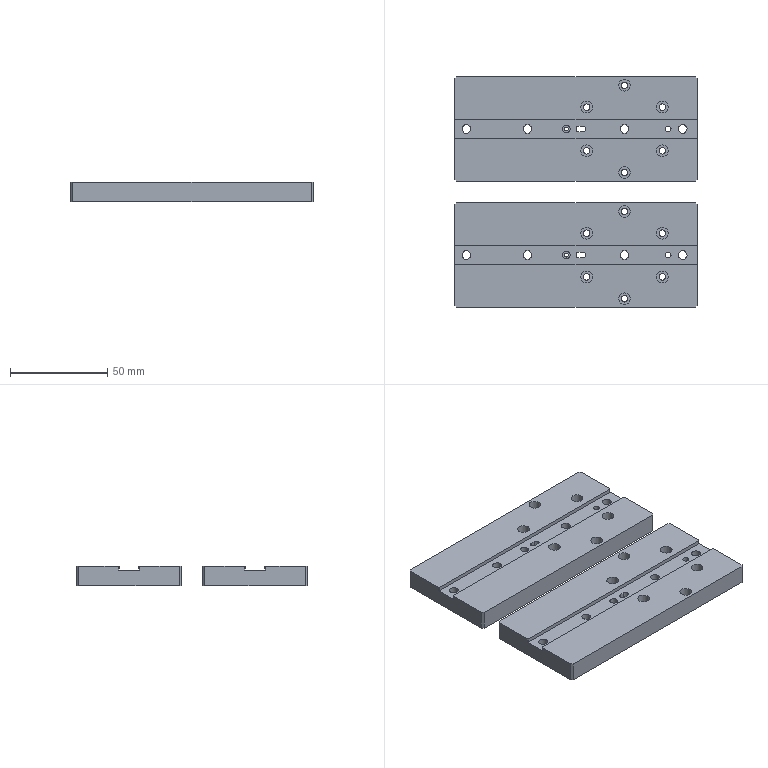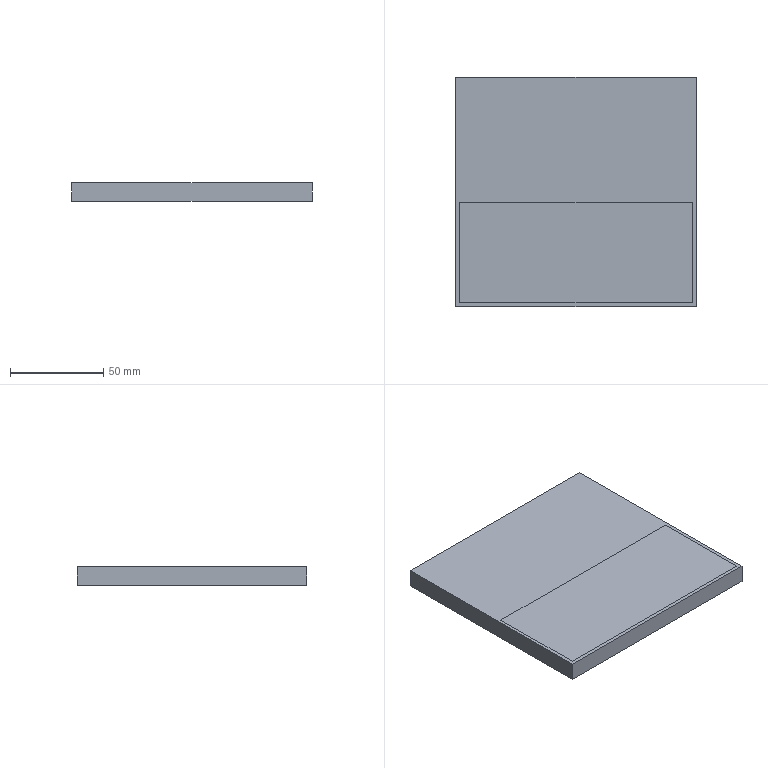CAM job | NX | 3-axis milling, drilling | part box 125 x 119 x 10 mm | stock box 129 x 123 x 10 mm
Tools:
number,name,description,diameter,corner_radius,flute_length,length,flutes
22,D6A45,Milling Tool-5 Parameters,6.0,0.0,3.0,3.0,2
20,D10,Milling Tool-5 Parameters,10.0,0.0,50.0,75.0,2
15,D4,Milling Tool-5 Parameters,4.0,0.0,50.0,75.0,2
13,D3,Milling Tool-5 Parameters,3.0,0.0,50.0,75.0,2
11,D10JING,Milling Tool-5 Parameters,10.0,0.0,50.0,75.0,2
19,4.5ZT,Drilling Tool,4.5,0.0,35.0,50.0,2
21,3.4ZT,Drilling Tool,3.4,0.0,35.0,50.0,2
24,2.0ZT,Drilling Tool,2.0,0.0,35.0,50.0,2
17,D6,Milling Tool-5 Parameters,6.0,0.0,50.0,75.0,2
12,D2,Milling Tool-5 Parameters,2.0,0.0,50.0,75.0,2
Operations:
program,operation,operation_type,tool,method,geometry_group,spindle_rpm,surface_speed,feed_per_tooth,feed_cut,feed_plunge,cut_length_mm,path_length_mm,cut_time_min,machine_time_min
1AB胶-130-125-10毛胚,DRILLING_COPY_1_COPY_1,Operation,D6A45,METHOD,A,5000.0,94.0,0.025,250.0,0.0,104.0,798.794,0.416,0.4855
1AB胶-130-125-10毛胚,DRILLING_COPY_1_COPY_COPY_COPY_COPY_1_COPY_COPY_1,Operation,4.5ZT,METHOD,A,2000.0,20.0,0.0375,150.0,0.0,122.816,615.464,0.8188,0.868
1AB胶-130-125-10毛胚,DRILLING_COPY_1_COPY_COPY_COPY_COPY_1_COPY_COPY_1_COPY,Operation,3.4ZT,METHOD,A,2000.0,20.0,0.0375,150.0,0.0,180.258,700.804,1.202,1.254
1AB胶-130-125-10毛胚,DRILLING_COPY_1_COPY_COPY_COPY_COPY_1_COPY_COPY_1_COPY_COPY,Operation,2.0ZT,METHOD,A,2000.0,20.0,0.0375,150.0,0.0,87.605,421.512,0.584,0.6174
1AB胶-130-125-10毛胚,ZLEVEL_PROFILE_COPY,ZLevelMilling,D10,METHOD,A,7500.0,235.0,0.1667,2500.0,100.0,7958.118,8205.184,3.183,3.208
1AB胶-130-125-10毛胚,FLOOR_WALL,VolumeBased25DMillingOperation,D6,METHOD,A,9500.0,179.0,0.0947,1800.0,100.0,2230.497,2460.506,1.239,1.262
1AB胶-130-125-10毛胚,HOLE_MILLING_COPY,CylinderMilling,D4,METHOD,A,7500.0,141.0,0.0933,1400.0,100.0,1340.799,2388.34,0.9577,1.062
1AB胶-130-125-10毛胚,HOLE_MILLING_COPY_COPY,CylinderMilling,D3,METHOD,A,7500.0,70.0,0.0867,1300.0,100.0,171.419,375.419,0.1319,0.1523
1AB胶-130-125-10毛胚,ZLEVEL_PROFILE_COPY_COPY,ZLevelMilling,D2,METHOD,A,7500.0,47.0,0.0667,1000.0,100.0,1035.279,1474.899,1.035,1.079
1AB胶-130-125-10毛胚,ZLEVEL_PROFILE_1_COPY_1_COPY_COPY,ZLevelMilling,D6A45,METHOD,A,7500.0,141.0,0.0667,1000.0,100.0,1429.777,2928.989,1.43,1.58
1AB胶-130-125-10毛胚,刀补13,CylinderMilling,D3,METHOD,A,7500.0,70.0,0.0667,1000.0,100.0,47.44,251.44,0.0474,0.0678
1AB胶-130-125-10毛胚,刀补12_1,ZLevelMilling,D2,METHOD,A,7500.0,47.0,0.0667,1000.0,100.0,146.58,587.06,0.1466,0.1906
1AB胶-130-125-10毛胚,刀补6,VolumeBased25DMillingOperation,D6,METHOD,A,9500.0,179.0,0.0526,1000.0,100.0,562.4,743.333,0.5624,0.5805
1AB胶-130-125-10毛胚,ZLEVEL_PROFILE_COPY_COPY_1,ZLevelMilling,D10JING,METHOD,A,7500.0,235.0,0.0667,1000.0,100.0,2403.136,2713.508,2.403,2.434
2,HOLE_MILLING_COPY_COPY_1,CylinderMilling,D6,METHOD,B,7500.0,141.0,0.0933,1400.0,100.0,358.79,726.69,0.2563,0.2931
2,ZLEVEL_PROFILE_1_COPY_1_COPY_COPY_COPY,ZLevelMilling,D6A45,METHOD,B,7500.0,141.0,0.0667,1000.0,100.0,538.396,1955.533,0.5384,0.6801